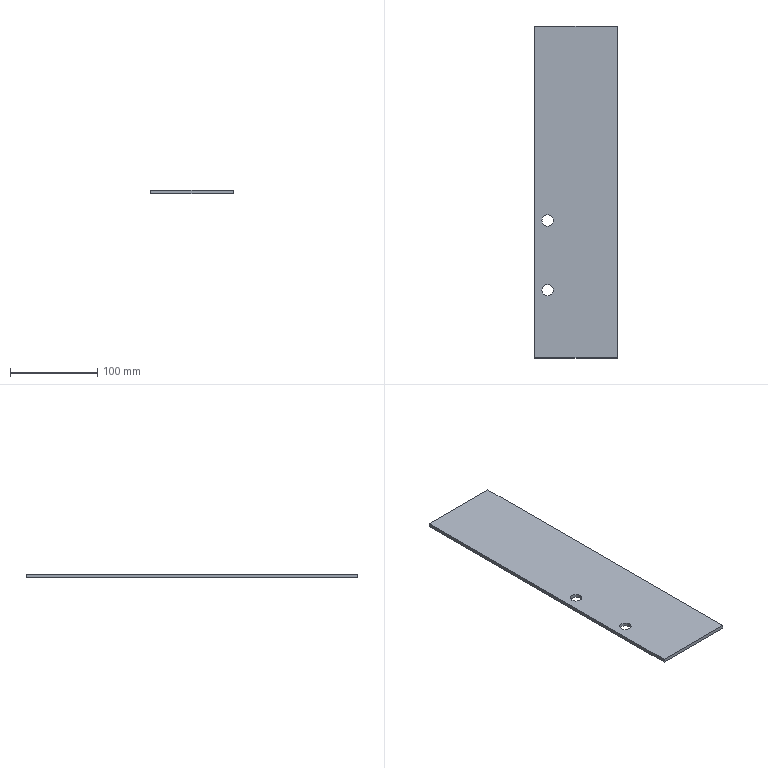Part | SolidWorks | features Extrusion 1 | 1 solid | 10 faces | box 95 x 380 x 4 mm | volume 143338 mm3 | plane 6 | cylinder 4 | commonest cylinder face diameters 13 x4
STEP:
#1=CARTESIAN_POINT('',(8.5,-222.5,4.));
#2=VERTEX_POINT('',#1);
#3=CARTESIAN_POINT('',(21.5,-222.5,4.));
#4=VERTEX_POINT('',#3);
#5=CARTESIAN_POINT('',(15.,-222.5,4.));
#6=DIRECTION('',(0.,0.,1.));
#7=DIRECTION('',(1.,0.,0.));
#8=AXIS2_PLACEMENT_3D('',#5,#6,#7);
#9=CIRCLE('',#8,6.5);
#10=EDGE_CURVE('',#2,#4,#9,.T.);
#11=ORIENTED_EDGE('',*,*,#10,.T.);
#12=CARTESIAN_POINT('',(21.5,-222.5,0.));
#13=VERTEX_POINT('',#12);
#14=CARTESIAN_POINT('',(21.5,-222.5,4.));
#15=DIRECTION('',(0.,0.,-1.));
#16=VECTOR('',#15,1000.);
#17=LINE('',#14,#16);
#18=EDGE_CURVE('',#4,#13,#17,.T.);
#19=ORIENTED_EDGE('',*,*,#18,.T.);
#20=CARTESIAN_POINT('',(8.5,-222.5,0.));
#21=VERTEX_POINT('',#20);
#22=CARTESIAN_POINT('',(15.,-222.5,0.));
#23=DIRECTION('',(0.,0.,1.));
#24=DIRECTION('',(1.,0.,0.));
#25=AXIS2_PLACEMENT_3D('',#22,#23,#24);
#26=CIRCLE('',#25,6.5);
#27=EDGE_CURVE('',#21,#13,#26,.T.);
#28=ORIENTED_EDGE('',*,*,#27,.F.);
#29=CARTESIAN_POINT('',(8.5,-222.5,4.));
#30=DIRECTION('',(0.,0.,-1.));
#31=VECTOR('',#30,1000.);
#32=LINE('',#29,#31);
#33=EDGE_CURVE('',#2,#21,#32,.T.);
#34=ORIENTED_EDGE('',*,*,#33,.F.);
#35=EDGE_LOOP('',(#11,#19,#28,#34));
#36=FACE_OUTER_BOUND('',#35,.T.);
#37=CARTESIAN_POINT('',(15.,-222.5,4.));
#38=DIRECTION('',(0.,0.,-1.));
#39=DIRECTION('',(-1.,0.,0.));
#40=AXIS2_PLACEMENT_3D('',#37,#38,#39);
#41=CYLINDRICAL_SURFACE('',#40,6.5);
#42=ADVANCED_FACE('',(#36),#41,.F.);
#43=CARTESIAN_POINT('',(8.5,-302.5,4.));
#44=VERTEX_POINT('',#43);
#45=CARTESIAN_POINT('',(21.5,-302.5,4.));
#46=VERTEX_POINT('',#45);
#47=CARTESIAN_POINT('',(15.,-302.5,4.));
#48=DIRECTION('',(0.,0.,1.));
#49=DIRECTION('',(1.,0.,0.));
#50=AXIS2_PLACEMENT_3D('',#47,#48,#49);
#51=CIRCLE('',#50,6.5);
#52=EDGE_CURVE('',#44,#46,#51,.T.);
#53=ORIENTED_EDGE('',*,*,#52,.T.);
#54=CARTESIAN_POINT('',(21.5,-302.5,0.));
#55=VERTEX_POINT('',#54);
#56=CARTESIAN_POINT('',(21.5,-302.5,4.));
#57=DIRECTION('',(0.,0.,-1.));
#58=VECTOR('',#57,1000.);
#59=LINE('',#56,#58);
#60=EDGE_CURVE('',#46,#55,#59,.T.);
#61=ORIENTED_EDGE('',*,*,#60,.T.);
#62=CARTESIAN_POINT('',(8.5,-302.5,0.));
#63=VERTEX_POINT('',#62);
#64=CARTESIAN_POINT('',(15.,-302.5,0.));
#65=DIRECTION('',(0.,0.,1.));
#66=DIRECTION('',(1.,0.,0.));
#67=AXIS2_PLACEMENT_3D('',#64,#65,#66);
#68=CIRCLE('',#67,6.5);
#69=EDGE_CURVE('',#63,#55,#68,.T.);
#70=ORIENTED_EDGE('',*,*,#69,.F.);
#71=CARTESIAN_POINT('',(8.5,-302.5,4.));
#72=DIRECTION('',(0.,0.,-1.));
#73=VECTOR('',#72,1000.);
#74=LINE('',#71,#73);
#75=EDGE_CURVE('',#44,#63,#74,.T.);
#76=ORIENTED_EDGE('',*,*,#75,.F.);
#77=EDGE_LOOP('',(#53,#61,#70,#76));
#78=FACE_OUTER_BOUND('',#77,.T.);
#79=CARTESIAN_POINT('',(15.,-302.5,4.));
#80=DIRECTION('',(0.,0.,-1.));
#81=DIRECTION('',(-1.,0.,0.));
#82=AXIS2_PLACEMENT_3D('',#79,#80,#81);
#83=CYLINDRICAL_SURFACE('',#82,6.5);
#84=ADVANCED_FACE('',(#78),#83,.F.);
#85=CARTESIAN_POINT('',(0.,0.,4.));
#86=VERTEX_POINT('',#85);
#87=CARTESIAN_POINT('',(0.,-380.,4.));
#88=VERTEX_POINT('',#87);
#89=CARTESIAN_POINT('',(0.,-380.,4.));
#90=DIRECTION('',(0.,-1.,0.));
#91=VECTOR('',#90,1000.);
#92=LINE('',#89,#91);
#93=EDGE_CURVE('',#86,#88,#92,.T.);
#94=ORIENTED_EDGE('',*,*,#93,.T.);
#95=CARTESIAN_POINT('',(95.,-380.,4.));
#96=VERTEX_POINT('',#95);
#97=CARTESIAN_POINT('',(95.,-380.,4.));
#98=DIRECTION('',(1.,0.,0.));
#99=VECTOR('',#98,1000.);
#100=LINE('',#97,#99);
#101=EDGE_CURVE('',#88,#96,#100,.T.);
#102=ORIENTED_EDGE('',*,*,#101,.T.);
#103=CARTESIAN_POINT('',(95.,0.,4.));
#104=VERTEX_POINT('',#103);
#105=CARTESIAN_POINT('',(95.,0.,4.));
#106=DIRECTION('',(0.,1.,0.));
#107=VECTOR('',#106,1000.);
#108=LINE('',#105,#107);
#109=EDGE_CURVE('',#96,#104,#108,.T.);
#110=ORIENTED_EDGE('',*,*,#109,.T.);
#111=CARTESIAN_POINT('',(0.,0.,4.));
#112=DIRECTION('',(-1.,0.,0.));
#113=VECTOR('',#112,1000.);
#114=LINE('',#111,#113);
#115=EDGE_CURVE('',#104,#86,#114,.T.);
#116=ORIENTED_EDGE('',*,*,#115,.T.);
#117=EDGE_LOOP('',(#94,#102,#110,#116));
#118=FACE_OUTER_BOUND('',#117,.T.);
#119=ORIENTED_EDGE('',*,*,#52,.F.);
#120=CARTESIAN_POINT('',(15.,-302.5,4.));
#121=DIRECTION('',(0.,0.,1.));
#122=DIRECTION('',(1.,0.,0.));
#123=AXIS2_PLACEMENT_3D('',#120,#121,#122);
#124=CIRCLE('',#123,6.5);
#125=EDGE_CURVE('',#46,#44,#124,.T.);
#126=ORIENTED_EDGE('',*,*,#125,.F.);
#127=EDGE_LOOP('',(#119,#126));
#128=FACE_BOUND('',#127,.T.);
#129=ORIENTED_EDGE('',*,*,#10,.F.);
#130=CARTESIAN_POINT('',(15.,-222.5,4.));
#131=DIRECTION('',(0.,0.,1.));
#132=DIRECTION('',(1.,0.,0.));
#133=AXIS2_PLACEMENT_3D('',#130,#131,#132);
#134=CIRCLE('',#133,6.5);
#135=EDGE_CURVE('',#4,#2,#134,.T.);
#136=ORIENTED_EDGE('',*,*,#135,.F.);
#137=EDGE_LOOP('',(#129,#136));
#138=FACE_BOUND('',#137,.T.);
#139=CARTESIAN_POINT('',(0.,0.,4.));
#140=DIRECTION('',(0.,0.,-1.));
#141=DIRECTION('',(-1.,0.,0.));
#142=AXIS2_PLACEMENT_3D('',#139,#140,#141);
#143=PLANE('',#142);
#144=ADVANCED_FACE('',(#118,#128,#138),#143,.F.);
#145=ORIENTED_EDGE('',*,*,#69,.T.);
#146=CARTESIAN_POINT('',(15.,-302.5,0.));
#147=DIRECTION('',(0.,0.,1.));
#148=DIRECTION('',(1.,0.,0.));
#149=AXIS2_PLACEMENT_3D('',#146,#147,#148);
#150=CIRCLE('',#149,6.5);
#151=EDGE_CURVE('',#55,#63,#150,.T.);
#152=ORIENTED_EDGE('',*,*,#151,.T.);
#153=EDGE_LOOP('',(#145,#152));
#154=FACE_BOUND('',#153,.T.);
#155=CARTESIAN_POINT('',(0.,0.,0.));
#156=VERTEX_POINT('',#155);
#157=CARTESIAN_POINT('',(0.,-380.,0.));
#158=VERTEX_POINT('',#157);
#159=CARTESIAN_POINT('',(0.,-380.,0.));
#160=DIRECTION('',(0.,-1.,0.));
#161=VECTOR('',#160,1000.);
#162=LINE('',#159,#161);
#163=EDGE_CURVE('',#156,#158,#162,.T.);
#164=ORIENTED_EDGE('',*,*,#163,.F.);
#165=CARTESIAN_POINT('',(95.,0.,0.));
#166=VERTEX_POINT('',#165);
#167=CARTESIAN_POINT('',(0.,0.,0.));
#168=DIRECTION('',(-1.,0.,0.));
#169=VECTOR('',#168,1000.);
#170=LINE('',#167,#169);
#171=EDGE_CURVE('',#166,#156,#170,.T.);
#172=ORIENTED_EDGE('',*,*,#171,.F.);
#173=CARTESIAN_POINT('',(95.,-380.,0.));
#174=VERTEX_POINT('',#173);
#175=CARTESIAN_POINT('',(95.,0.,0.));
#176=DIRECTION('',(0.,1.,0.));
#177=VECTOR('',#176,1000.);
#178=LINE('',#175,#177);
#179=EDGE_CURVE('',#174,#166,#178,.T.);
#180=ORIENTED_EDGE('',*,*,#179,.F.);
#181=CARTESIAN_POINT('',(95.,-380.,0.));
#182=DIRECTION('',(1.,0.,0.));
#183=VECTOR('',#182,1000.);
#184=LINE('',#181,#183);
#185=EDGE_CURVE('',#158,#174,#184,.T.);
#186=ORIENTED_EDGE('',*,*,#185,.F.);
#187=EDGE_LOOP('',(#164,#172,#180,#186));
#188=FACE_OUTER_BOUND('',#187,.T.);
#189=ORIENTED_EDGE('',*,*,#27,.T.);
#190=CARTESIAN_POINT('',(15.,-222.5,0.));
#191=DIRECTION('',(0.,0.,1.));
#192=DIRECTION('',(1.,0.,0.));
#193=AXIS2_PLACEMENT_3D('',#190,#191,#192);
#194=CIRCLE('',#193,6.5);
#195=EDGE_CURVE('',#13,#21,#194,.T.);
#196=ORIENTED_EDGE('',*,*,#195,.T.);
#197=EDGE_LOOP('',(#189,#196));
#198=FACE_BOUND('',#197,.T.);
#199=CARTESIAN_POINT('',(0.,0.,0.));
#200=DIRECTION('',(0.,0.,-1.));
#201=DIRECTION('',(-1.,0.,0.));
#202=AXIS2_PLACEMENT_3D('',#199,#200,#201);
#203=PLANE('',#202);
#204=ADVANCED_FACE('',(#154,#188,#198),#203,.T.);
#205=ORIENTED_EDGE('',*,*,#163,.T.);
#206=CARTESIAN_POINT('',(0.,-380.,4.));
#207=DIRECTION('',(0.,0.,-1.));
#208=VECTOR('',#207,1000.);
#209=LINE('',#206,#208);
#210=EDGE_CURVE('',#88,#158,#209,.T.);
#211=ORIENTED_EDGE('',*,*,#210,.F.);
#212=ORIENTED_EDGE('',*,*,#93,.F.);
#213=CARTESIAN_POINT('',(0.,0.,4.));
#214=DIRECTION('',(0.,0.,-1.));
#215=VECTOR('',#214,1000.);
#216=LINE('',#213,#215);
#217=EDGE_CURVE('',#86,#156,#216,.T.);
#218=ORIENTED_EDGE('',*,*,#217,.T.);
#219=EDGE_LOOP('',(#205,#211,#212,#218));
#220=FACE_OUTER_BOUND('',#219,.T.);
#221=CARTESIAN_POINT('',(0.,-380.,4.));
#222=DIRECTION('',(1.,0.,0.));
#223=DIRECTION('',(0.,0.,-1.));
#224=AXIS2_PLACEMENT_3D('',#221,#222,#223);
#225=PLANE('',#224);
#226=ADVANCED_FACE('',(#220),#225,.F.);
#227=ORIENTED_EDGE('',*,*,#185,.T.);
#228=CARTESIAN_POINT('',(95.,-380.,4.));
#229=DIRECTION('',(0.,0.,-1.));
#230=VECTOR('',#229,1000.);
#231=LINE('',#228,#230);
#232=EDGE_CURVE('',#96,#174,#231,.T.);
#233=ORIENTED_EDGE('',*,*,#232,.F.);
#234=ORIENTED_EDGE('',*,*,#101,.F.);
#235=ORIENTED_EDGE('',*,*,#210,.T.);
#236=EDGE_LOOP('',(#227,#233,#234,#235));
#237=FACE_OUTER_BOUND('',#236,.T.);
#238=CARTESIAN_POINT('',(95.,-380.,4.));
#239=DIRECTION('',(0.,1.,0.));
#240=DIRECTION('',(0.,0.,1.));
#241=AXIS2_PLACEMENT_3D('',#238,#239,#240);
#242=PLANE('',#241);
#243=ADVANCED_FACE('',(#237),#242,.F.);
#244=ORIENTED_EDGE('',*,*,#179,.T.);
#245=CARTESIAN_POINT('',(95.,0.,4.));
#246=DIRECTION('',(0.,0.,-1.));
#247=VECTOR('',#246,1000.);
#248=LINE('',#245,#247);
#249=EDGE_CURVE('',#104,#166,#248,.T.);
#250=ORIENTED_EDGE('',*,*,#249,.F.);
#251=ORIENTED_EDGE('',*,*,#109,.F.);
#252=ORIENTED_EDGE('',*,*,#232,.T.);
#253=EDGE_LOOP('',(#244,#250,#251,#252));
#254=FACE_OUTER_BOUND('',#253,.T.);
#255=CARTESIAN_POINT('',(95.,0.,4.));
#256=DIRECTION('',(-1.,0.,0.));
#257=DIRECTION('',(0.,-1.,0.));
#258=AXIS2_PLACEMENT_3D('',#255,#256,#257);
#259=PLANE('',#258);
#260=ADVANCED_FACE('',(#254),#259,.F.);
#261=ORIENTED_EDGE('',*,*,#171,.T.);
#262=ORIENTED_EDGE('',*,*,#217,.F.);
#263=ORIENTED_EDGE('',*,*,#115,.F.);
#264=ORIENTED_EDGE('',*,*,#249,.T.);
#265=EDGE_LOOP('',(#261,#262,#263,#264));
#266=FACE_OUTER_BOUND('',#265,.T.);
#267=CARTESIAN_POINT('',(0.,0.,4.));
#268=DIRECTION('',(0.,-1.,0.));
#269=DIRECTION('',(0.,0.,-1.));
#270=AXIS2_PLACEMENT_3D('',#267,#268,#269);
#271=PLANE('',#270);
#272=ADVANCED_FACE('',(#266),#271,.F.);
#273=ORIENTED_EDGE('',*,*,#60,.F.);
#274=ORIENTED_EDGE('',*,*,#125,.T.);
#275=ORIENTED_EDGE('',*,*,#75,.T.);
#276=ORIENTED_EDGE('',*,*,#151,.F.);
#277=EDGE_LOOP('',(#273,#274,#275,#276));
#278=FACE_OUTER_BOUND('',#277,.T.);
#279=CARTESIAN_POINT('',(15.,-302.5,4.));
#280=DIRECTION('',(0.,0.,-1.));
#281=DIRECTION('',(-1.,0.,0.));
#282=AXIS2_PLACEMENT_3D('',#279,#280,#281);
#283=CYLINDRICAL_SURFACE('',#282,6.5);
#284=ADVANCED_FACE('',(#278),#283,.F.);
#285=ORIENTED_EDGE('',*,*,#18,.F.);
#286=ORIENTED_EDGE('',*,*,#135,.T.);
#287=ORIENTED_EDGE('',*,*,#33,.T.);
#288=ORIENTED_EDGE('',*,*,#195,.F.);
#289=EDGE_LOOP('',(#285,#286,#287,#288));
#290=FACE_OUTER_BOUND('',#289,.T.);
#291=CARTESIAN_POINT('',(15.,-222.5,4.));
#292=DIRECTION('',(0.,0.,-1.));
#293=DIRECTION('',(-1.,0.,0.));
#294=AXIS2_PLACEMENT_3D('',#291,#292,#293);
#295=CYLINDRICAL_SURFACE('',#294,6.5);
#296=ADVANCED_FACE('',(#290),#295,.F.);
#297=CLOSED_SHELL('',(#42,#84,#144,#204,#226,#243,#260,#272,#284,#296));
#298=MANIFOLD_SOLID_BREP('',#297);
#299=CARTESIAN_POINT('',(0.,0.,0.));
#300=DIRECTION('',(0.,0.,1.));
#301=DIRECTION('',(1.,0.,0.));
#302=AXIS2_PLACEMENT_3D('',#299,#300,#301);
#303=(LENGTH_UNIT()NAMED_UNIT(*)SI_UNIT(.MILLI.,.METRE.));
#304=UNCERTAINTY_MEASURE_WITH_UNIT(LENGTH_MEASURE(0.00001),#303,'','');
#305=(NAMED_UNIT(*)PLANE_ANGLE_UNIT()SI_UNIT($,.RADIAN.));
#306=(NAMED_UNIT(*)SI_UNIT($,.STERADIAN.)SOLID_ANGLE_UNIT());
#307=(GEOMETRIC_REPRESENTATION_CONTEXT(3)GLOBAL_UNCERTAINTY_ASSIGNED_CONTEXT((#304))GLOBAL_UNIT_ASSIGNED_CONTEXT((#303,#305,#306))REPRESENTATION_CONTEXT('',''));
#308=ADVANCED_BREP_SHAPE_REPRESENTATION('',(#298,#302),#307);